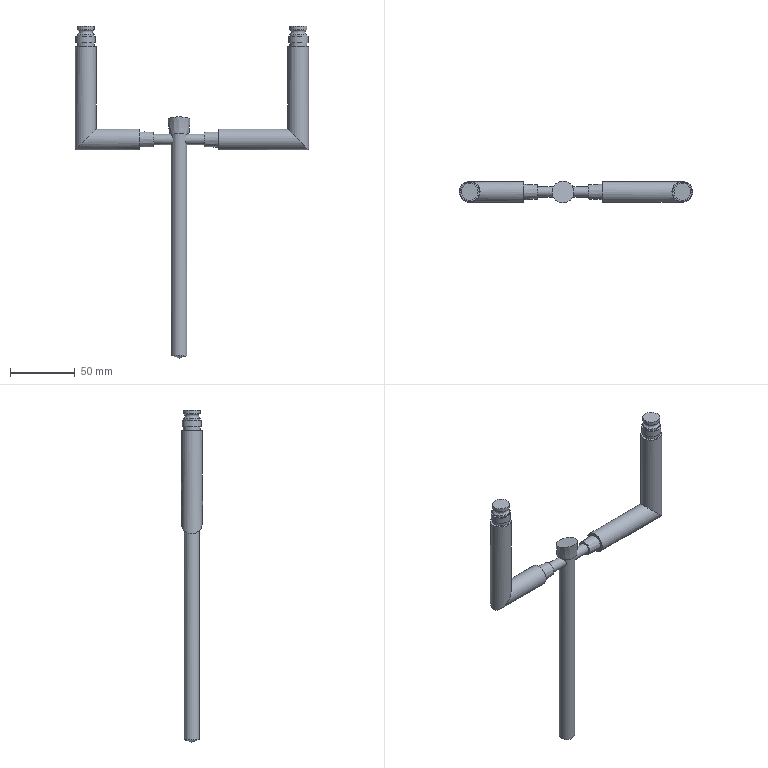Part | STEP file | COOLING-SLIDE2_id162_x_t | 1 solid | 35 faces | box 180 x 16.813 x 255.984 mm | volume 79230 mm3 | cylinder 15 | plane 14 | cone 4 | other 2 | commonest cylinder face diameters 13 x6 16 x4 8 x2 15 x2 12 x1
STEP:
#1=CARTESIAN_POINT('',(-95.5,0.,291.));
#2=VERTEX_POINT('',#1);
#3=CARTESIAN_POINT('',(-102.,0.,291.));
#4=DIRECTION('',(0.,0.,-1.));
#5=DIRECTION('',(1.,0.,0.));
#6=AXIS2_PLACEMENT_3D('',#3,#4,#5);
#7=CIRCLE('',#6,6.5);
#8=EDGE_CURVE('',#2,#2,#7,.T.);
#9=ORIENTED_EDGE('',*,*,#8,.F.);
#10=EDGE_LOOP('',(#9));
#11=FACE_OUTER_BOUND('',#10,.T.);
#12=CARTESIAN_POINT('',(-102.,0.,291.));
#13=DIRECTION('',(0.,0.,1.));
#14=DIRECTION('',(1.,0.,0.));
#15=AXIS2_PLACEMENT_3D('',#12,#13,#14);
#16=PLANE('',#15);
#17=ADVANCED_FACE('',(#11),#16,.T.);
#18=CARTESIAN_POINT('',(55.5,0.,291.));
#19=VERTEX_POINT('',#18);
#20=CARTESIAN_POINT('',(62.,0.,291.));
#21=DIRECTION('',(0.,0.,-1.));
#22=DIRECTION('',(-1.,0.,0.));
#23=AXIS2_PLACEMENT_3D('',#20,#21,#22);
#24=CIRCLE('',#23,6.5);
#25=EDGE_CURVE('',#19,#19,#24,.T.);
#26=ORIENTED_EDGE('',*,*,#25,.F.);
#27=EDGE_LOOP('',(#26));
#28=FACE_OUTER_BOUND('',#27,.T.);
#29=CARTESIAN_POINT('',(62.,0.,291.));
#30=DIRECTION('',(0.,0.,-1.));
#31=DIRECTION('',(-1.,0.,0.));
#32=AXIS2_PLACEMENT_3D('',#29,#30,#31);
#33=PLANE('',#32);
#34=ADVANCED_FACE('',(#28),#33,.F.);
#35=ORIENTED_EDGE('',*,*,#8,.T.);
#36=EDGE_LOOP('',(#35));
#37=FACE_BOUND('',#36,.T.);
#38=CARTESIAN_POINT('',(-108.5,0.,288.149));
#39=VERTEX_POINT('',#38);
#40=CARTESIAN_POINT('',(-102.,0.,288.149));
#41=DIRECTION('',(0.,0.,1.));
#42=DIRECTION('',(-1.,0.,0.));
#43=AXIS2_PLACEMENT_3D('',#40,#41,#42);
#44=CIRCLE('',#43,6.5);
#45=EDGE_CURVE('',#39,#39,#44,.T.);
#46=ORIENTED_EDGE('',*,*,#45,.T.);
#47=EDGE_LOOP('',(#46));
#48=FACE_BOUND('',#47,.T.);
#49=CARTESIAN_POINT('',(-102.,0.,190.725));
#50=DIRECTION('',(0.,0.,1.));
#51=DIRECTION('',(1.,0.,0.));
#52=AXIS2_PLACEMENT_3D('',#49,#50,#51);
#53=CYLINDRICAL_SURFACE('',#52,6.5);
#54=ADVANCED_FACE('',(#37,#48),#53,.T.);
#55=CARTESIAN_POINT('',(68.5,0.,288.149));
#56=VERTEX_POINT('',#55);
#57=CARTESIAN_POINT('',(62.,0.,288.149));
#58=DIRECTION('',(0.,0.,1.));
#59=DIRECTION('',(1.,0.,0.));
#60=AXIS2_PLACEMENT_3D('',#57,#58,#59);
#61=CIRCLE('',#60,6.5);
#62=EDGE_CURVE('',#56,#56,#61,.T.);
#63=ORIENTED_EDGE('',*,*,#62,.T.);
#64=EDGE_LOOP('',(#63));
#65=FACE_BOUND('',#64,.T.);
#66=ORIENTED_EDGE('',*,*,#25,.T.);
#67=EDGE_LOOP('',(#66));
#68=FACE_BOUND('',#67,.T.);
#69=CARTESIAN_POINT('',(62.,0.,295.775));
#70=DIRECTION('',(0.,0.,-1.));
#71=DIRECTION('',(-1.,0.,0.));
#72=AXIS2_PLACEMENT_3D('',#69,#70,#71);
#73=CYLINDRICAL_SURFACE('',#72,6.5);
#74=ADVANCED_FACE('',(#65,#68),#73,.T.);
#75=ORIENTED_EDGE('',*,*,#45,.F.);
#76=EDGE_LOOP('',(#75));
#77=FACE_BOUND('',#76,.T.);
#78=CARTESIAN_POINT('',(-95.5,0.,284.433));
#79=VERTEX_POINT('',#78);
#80=CARTESIAN_POINT('',(-102.,0.,284.433));
#81=DIRECTION('',(0.,0.,-1.));
#82=DIRECTION('',(1.,0.,0.));
#83=AXIS2_PLACEMENT_3D('',#80,#81,#82);
#84=CIRCLE('',#83,6.5);
#85=EDGE_CURVE('',#79,#79,#84,.T.);
#86=ORIENTED_EDGE('',*,*,#85,.F.);
#87=EDGE_LOOP('',(#86));
#88=FACE_BOUND('',#87,.T.);
#89=CARTESIAN_POINT('',(-109.241,0.,286.291));
#90=DIRECTION('',(0.,-1.,0.));
#91=DIRECTION('',(-1.,0.,0.));
#92=AXIS2_PLACEMENT_3D('',#89,#90,#91);
#93=CIRCLE('',#92,2.);
#94=CARTESIAN_POINT('',(-102.,0.,286.291));
#95=DIRECTION('',(0.,0.,1.));
#96=AXIS1_PLACEMENT('',#94,#95);
#97=SURFACE_OF_REVOLUTION('',#93,#96);
#98=ADVANCED_FACE('',(#77,#88),#97,.T.);
#99=CARTESIAN_POINT('',(55.5,0.,284.433));
#100=VERTEX_POINT('',#99);
#101=CARTESIAN_POINT('',(62.,0.,284.433));
#102=DIRECTION('',(0.,0.,-1.));
#103=DIRECTION('',(-1.,0.,0.));
#104=AXIS2_PLACEMENT_3D('',#101,#102,#103);
#105=CIRCLE('',#104,6.5);
#106=EDGE_CURVE('',#100,#100,#105,.T.);
#107=ORIENTED_EDGE('',*,*,#106,.F.);
#108=EDGE_LOOP('',(#107));
#109=FACE_BOUND('',#108,.T.);
#110=ORIENTED_EDGE('',*,*,#62,.F.);
#111=EDGE_LOOP('',(#110));
#112=FACE_BOUND('',#111,.T.);
#113=CARTESIAN_POINT('',(69.241,0.,286.291));
#114=DIRECTION('',(0.,-1.,0.));
#115=DIRECTION('',(1.,0.,0.));
#116=AXIS2_PLACEMENT_3D('',#113,#114,#115);
#117=CIRCLE('',#116,2.);
#118=CARTESIAN_POINT('',(62.,0.,286.291));
#119=DIRECTION('',(0.,0.,-1.));
#120=AXIS1_PLACEMENT('',#118,#119);
#121=SURFACE_OF_REVOLUTION('',#117,#120);
#122=ADVANCED_FACE('',(#109,#112),#121,.T.);
#123=ORIENTED_EDGE('',*,*,#85,.T.);
#124=EDGE_LOOP('',(#123));
#125=FACE_BOUND('',#124,.T.);
#126=CARTESIAN_POINT('',(-95.5,0.,283.));
#127=VERTEX_POINT('',#126);
#128=CARTESIAN_POINT('',(-102.,0.,283.));
#129=DIRECTION('',(0.,0.,-1.));
#130=DIRECTION('',(1.,0.,0.));
#131=AXIS2_PLACEMENT_3D('',#128,#129,#130);
#132=CIRCLE('',#131,6.5);
#133=EDGE_CURVE('',#127,#127,#132,.T.);
#134=ORIENTED_EDGE('',*,*,#133,.F.);
#135=EDGE_LOOP('',(#134));
#136=FACE_BOUND('',#135,.T.);
#137=CARTESIAN_POINT('',(-102.,0.,190.725));
#138=DIRECTION('',(0.,0.,1.));
#139=DIRECTION('',(1.,0.,0.));
#140=AXIS2_PLACEMENT_3D('',#137,#138,#139);
#141=CYLINDRICAL_SURFACE('',#140,6.5);
#142=ADVANCED_FACE('',(#125,#136),#141,.T.);
#143=CARTESIAN_POINT('',(55.5,0.,283.));
#144=VERTEX_POINT('',#143);
#145=CARTESIAN_POINT('',(62.,0.,283.));
#146=DIRECTION('',(0.,0.,1.));
#147=DIRECTION('',(-1.,0.,0.));
#148=AXIS2_PLACEMENT_3D('',#145,#146,#147);
#149=CIRCLE('',#148,6.5);
#150=EDGE_CURVE('',#144,#144,#149,.T.);
#151=ORIENTED_EDGE('',*,*,#150,.T.);
#152=EDGE_LOOP('',(#151));
#153=FACE_BOUND('',#152,.T.);
#154=ORIENTED_EDGE('',*,*,#106,.T.);
#155=EDGE_LOOP('',(#154));
#156=FACE_BOUND('',#155,.T.);
#157=CARTESIAN_POINT('',(62.,0.,295.775));
#158=DIRECTION('',(0.,0.,-1.));
#159=DIRECTION('',(-1.,0.,0.));
#160=AXIS2_PLACEMENT_3D('',#157,#158,#159);
#161=CYLINDRICAL_SURFACE('',#160,6.5);
#162=ADVANCED_FACE('',(#153,#156),#161,.T.);
#163=ORIENTED_EDGE('',*,*,#133,.T.);
#164=EDGE_LOOP('',(#163));
#165=FACE_BOUND('',#164,.T.);
#166=CARTESIAN_POINT('',(-94.5,0.,283.));
#167=VERTEX_POINT('',#166);
#168=CARTESIAN_POINT('',(-102.,0.,283.));
#169=DIRECTION('',(0.,0.,-1.));
#170=DIRECTION('',(1.,0.,0.));
#171=AXIS2_PLACEMENT_3D('',#168,#169,#170);
#172=CIRCLE('',#171,7.5);
#173=EDGE_CURVE('',#167,#167,#172,.T.);
#174=ORIENTED_EDGE('',*,*,#173,.F.);
#175=EDGE_LOOP('',(#174));
#176=FACE_BOUND('',#175,.T.);
#177=CARTESIAN_POINT('',(-102.,0.,283.));
#178=DIRECTION('',(0.,0.,1.));
#179=DIRECTION('',(1.,0.,0.));
#180=AXIS2_PLACEMENT_3D('',#177,#178,#179);
#181=PLANE('',#180);
#182=ADVANCED_FACE('',(#165,#176),#181,.T.);
#183=ORIENTED_EDGE('',*,*,#150,.F.);
#184=EDGE_LOOP('',(#183));
#185=FACE_BOUND('',#184,.T.);
#186=CARTESIAN_POINT('',(54.5,0.,283.));
#187=VERTEX_POINT('',#186);
#188=CARTESIAN_POINT('',(62.,0.,283.));
#189=DIRECTION('',(0.,0.,-1.));
#190=DIRECTION('',(-1.,0.,0.));
#191=AXIS2_PLACEMENT_3D('',#188,#189,#190);
#192=CIRCLE('',#191,7.5);
#193=EDGE_CURVE('',#187,#187,#192,.T.);
#194=ORIENTED_EDGE('',*,*,#193,.F.);
#195=EDGE_LOOP('',(#194));
#196=FACE_BOUND('',#195,.T.);
#197=CARTESIAN_POINT('',(62.,0.,283.));
#198=DIRECTION('',(0.,0.,-1.));
#199=DIRECTION('',(-1.,0.,0.));
#200=AXIS2_PLACEMENT_3D('',#197,#198,#199);
#201=PLANE('',#200);
#202=ADVANCED_FACE('',(#185,#196),#201,.F.);
#203=CARTESIAN_POINT('',(-94.5,0.,278.));
#204=VERTEX_POINT('',#203);
#205=CARTESIAN_POINT('',(-102.,0.,278.));
#206=DIRECTION('',(0.,0.,1.));
#207=DIRECTION('',(1.,0.,0.));
#208=AXIS2_PLACEMENT_3D('',#205,#206,#207);
#209=CIRCLE('',#208,7.5);
#210=EDGE_CURVE('',#204,#204,#209,.T.);
#211=ORIENTED_EDGE('',*,*,#210,.T.);
#212=EDGE_LOOP('',(#211));
#213=FACE_BOUND('',#212,.T.);
#214=ORIENTED_EDGE('',*,*,#173,.T.);
#215=EDGE_LOOP('',(#214));
#216=FACE_BOUND('',#215,.T.);
#217=CARTESIAN_POINT('',(-102.,0.,190.725));
#218=DIRECTION('',(0.,0.,1.));
#219=DIRECTION('',(1.,0.,0.));
#220=AXIS2_PLACEMENT_3D('',#217,#218,#219);
#221=CYLINDRICAL_SURFACE('',#220,7.5);
#222=ADVANCED_FACE('',(#213,#216),#221,.T.);
#223=ORIENTED_EDGE('',*,*,#193,.T.);
#224=EDGE_LOOP('',(#223));
#225=FACE_BOUND('',#224,.T.);
#226=CARTESIAN_POINT('',(54.5,0.,278.));
#227=VERTEX_POINT('',#226);
#228=CARTESIAN_POINT('',(62.,0.,278.));
#229=DIRECTION('',(0.,0.,-1.));
#230=DIRECTION('',(-1.,0.,0.));
#231=AXIS2_PLACEMENT_3D('',#228,#229,#230);
#232=CIRCLE('',#231,7.5);
#233=EDGE_CURVE('',#227,#227,#232,.T.);
#234=ORIENTED_EDGE('',*,*,#233,.F.);
#235=EDGE_LOOP('',(#234));
#236=FACE_BOUND('',#235,.T.);
#237=CARTESIAN_POINT('',(62.,0.,295.775));
#238=DIRECTION('',(0.,0.,-1.));
#239=DIRECTION('',(-1.,0.,0.));
#240=AXIS2_PLACEMENT_3D('',#237,#238,#239);
#241=CYLINDRICAL_SURFACE('',#240,7.5);
#242=ADVANCED_FACE('',(#225,#236),#241,.T.);
#243=CARTESIAN_POINT('',(-95.5,0.,278.));
#244=VERTEX_POINT('',#243);
#245=CARTESIAN_POINT('',(-102.,0.,278.));
#246=DIRECTION('',(0.,0.,-1.));
#247=DIRECTION('',(1.,0.,0.));
#248=AXIS2_PLACEMENT_3D('',#245,#246,#247);
#249=CIRCLE('',#248,6.5);
#250=EDGE_CURVE('',#244,#244,#249,.T.);
#251=ORIENTED_EDGE('',*,*,#250,.F.);
#252=EDGE_LOOP('',(#251));
#253=FACE_BOUND('',#252,.T.);
#254=ORIENTED_EDGE('',*,*,#210,.F.);
#255=EDGE_LOOP('',(#254));
#256=FACE_BOUND('',#255,.T.);
#257=CARTESIAN_POINT('',(-102.,0.,278.));
#258=DIRECTION('',(0.,0.,1.));
#259=DIRECTION('',(1.,0.,0.));
#260=AXIS2_PLACEMENT_3D('',#257,#258,#259);
#261=PLANE('',#260);
#262=ADVANCED_FACE('',(#253,#256),#261,.F.);
#263=CARTESIAN_POINT('',(55.5,0.,278.));
#264=VERTEX_POINT('',#263);
#265=CARTESIAN_POINT('',(62.,0.,278.));
#266=DIRECTION('',(0.,0.,-1.));
#267=DIRECTION('',(-1.,0.,0.));
#268=AXIS2_PLACEMENT_3D('',#265,#266,#267);
#269=CIRCLE('',#268,6.5);
#270=EDGE_CURVE('',#264,#264,#269,.T.);
#271=ORIENTED_EDGE('',*,*,#270,.F.);
#272=EDGE_LOOP('',(#271));
#273=FACE_BOUND('',#272,.T.);
#274=ORIENTED_EDGE('',*,*,#233,.T.);
#275=EDGE_LOOP('',(#274));
#276=FACE_BOUND('',#275,.T.);
#277=CARTESIAN_POINT('',(62.,0.,278.));
#278=DIRECTION('',(0.,0.,-1.));
#279=DIRECTION('',(-1.,0.,0.));
#280=AXIS2_PLACEMENT_3D('',#277,#278,#279);
#281=PLANE('',#280);
#282=ADVANCED_FACE('',(#273,#276),#281,.T.);
#283=ORIENTED_EDGE('',*,*,#250,.T.);
#284=EDGE_LOOP('',(#283));
#285=FACE_BOUND('',#284,.T.);
#286=CARTESIAN_POINT('',(-95.5,0.,275.));
#287=VERTEX_POINT('',#286);
#288=CARTESIAN_POINT('',(-102.,0.,275.));
#289=DIRECTION('',(0.,0.,-1.));
#290=DIRECTION('',(1.,0.,0.));
#291=AXIS2_PLACEMENT_3D('',#288,#289,#290);
#292=CIRCLE('',#291,6.5);
#293=EDGE_CURVE('',#287,#287,#292,.T.);
#294=ORIENTED_EDGE('',*,*,#293,.F.);
#295=EDGE_LOOP('',(#294));
#296=FACE_BOUND('',#295,.T.);
#297=CARTESIAN_POINT('',(-102.,0.,190.725));
#298=DIRECTION('',(0.,0.,1.));
#299=DIRECTION('',(1.,0.,0.));
#300=AXIS2_PLACEMENT_3D('',#297,#298,#299);
#301=CYLINDRICAL_SURFACE('',#300,6.5);
#302=ADVANCED_FACE('',(#285,#296),#301,.T.);
#303=CARTESIAN_POINT('',(55.5,0.,275.));
#304=VERTEX_POINT('',#303);
#305=CARTESIAN_POINT('',(62.,0.,275.));
#306=DIRECTION('',(0.,0.,1.));
#307=DIRECTION('',(-1.,0.,0.));
#308=AXIS2_PLACEMENT_3D('',#305,#306,#307);
#309=CIRCLE('',#308,6.5);
#310=EDGE_CURVE('',#304,#304,#309,.T.);
#311=ORIENTED_EDGE('',*,*,#310,.T.);
#312=EDGE_LOOP('',(#311));
#313=FACE_BOUND('',#312,.T.);
#314=ORIENTED_EDGE('',*,*,#270,.T.);
#315=EDGE_LOOP('',(#314));
#316=FACE_BOUND('',#315,.T.);
#317=CARTESIAN_POINT('',(62.,0.,295.775));
#318=DIRECTION('',(0.,0.,-1.));
#319=DIRECTION('',(-1.,0.,0.));
#320=AXIS2_PLACEMENT_3D('',#317,#318,#319);
#321=CYLINDRICAL_SURFACE('',#320,6.5);
#322=ADVANCED_FACE('',(#313,#316),#321,.T.);
#323=ORIENTED_EDGE('',*,*,#293,.T.);
#324=EDGE_LOOP('',(#323));
#325=FACE_BOUND('',#324,.T.);
#326=CARTESIAN_POINT('',(-94.,0.,275.));
#327=VERTEX_POINT('',#326);
#328=CARTESIAN_POINT('',(-102.,0.,275.));
#329=DIRECTION('',(0.,0.,-1.));
#330=DIRECTION('',(1.,0.,0.));
#331=AXIS2_PLACEMENT_3D('',#328,#329,#330);
#332=CIRCLE('',#331,8.);
#333=EDGE_CURVE('',#327,#327,#332,.T.);
#334=ORIENTED_EDGE('',*,*,#333,.F.);
#335=EDGE_LOOP('',(#334));
#336=FACE_BOUND('',#335,.T.);
#337=CARTESIAN_POINT('',(-102.,0.,275.));
#338=DIRECTION('',(0.,0.,1.));
#339=DIRECTION('',(1.,0.,0.));
#340=AXIS2_PLACEMENT_3D('',#337,#338,#339);
#341=PLANE('',#340);
#342=ADVANCED_FACE('',(#325,#336),#341,.T.);
#343=ORIENTED_EDGE('',*,*,#310,.F.);
#344=EDGE_LOOP('',(#343));
#345=FACE_BOUND('',#344,.T.);
#346=CARTESIAN_POINT('',(54.,0.,275.));
#347=VERTEX_POINT('',#346);
#348=CARTESIAN_POINT('',(62.,0.,275.));
#349=DIRECTION('',(0.,0.,-1.));
#350=DIRECTION('',(-1.,0.,0.));
#351=AXIS2_PLACEMENT_3D('',#348,#349,#350);
#352=CIRCLE('',#351,8.);
#353=EDGE_CURVE('',#347,#347,#352,.T.);
#354=ORIENTED_EDGE('',*,*,#353,.F.);
#355=EDGE_LOOP('',(#354));
#356=FACE_BOUND('',#355,.T.);
#357=CARTESIAN_POINT('',(62.,0.,275.));
#358=DIRECTION('',(0.,0.,-1.));
#359=DIRECTION('',(-1.,0.,0.));
#360=AXIS2_PLACEMENT_3D('',#357,#358,#359);
#361=PLANE('',#360);
#362=ADVANCED_FACE('',(#345,#356),#361,.F.);
#363=ORIENTED_EDGE('',*,*,#333,.T.);
#364=EDGE_LOOP('',(#363));
#365=FACE_BOUND('',#364,.T.);
#366=CARTESIAN_POINT('',(-110.,0.,195.5));
#367=VERTEX_POINT('',#366);
#368=CARTESIAN_POINT('',(-102.,0.,203.5));
#369=DIRECTION('',(0.7071,0.,-0.7071));
#370=DIRECTION('',(-0.7071,0.,-0.7071));
#371=AXIS2_PLACEMENT_3D('',#368,#369,#370);
#372=ELLIPSE('',#371,11.314,8.);
#373=EDGE_CURVE('',#367,#367,#372,.T.);
#374=ORIENTED_EDGE('',*,*,#373,.F.);
#375=EDGE_LOOP('',(#374));
#376=FACE_BOUND('',#375,.T.);
#377=CARTESIAN_POINT('',(-102.,0.,190.725));
#378=DIRECTION('',(0.,0.,1.));
#379=DIRECTION('',(1.,0.,0.));
#380=AXIS2_PLACEMENT_3D('',#377,#378,#379);
#381=CYLINDRICAL_SURFACE('',#380,8.);
#382=ADVANCED_FACE('',(#365,#376),#381,.T.);
#383=ORIENTED_EDGE('',*,*,#353,.T.);
#384=EDGE_LOOP('',(#383));
#385=FACE_BOUND('',#384,.T.);
#386=CARTESIAN_POINT('',(54.,0.,211.5));
#387=VERTEX_POINT('',#386);
#388=CARTESIAN_POINT('',(62.,0.,203.5));
#389=DIRECTION('',(-0.7071,0.,-0.7071));
#390=DIRECTION('',(-0.7071,0.,0.7071));
#391=AXIS2_PLACEMENT_3D('',#388,#389,#390);
#392=ELLIPSE('',#391,11.314,8.);
#393=EDGE_CURVE('',#387,#387,#392,.T.);
#394=ORIENTED_EDGE('',*,*,#393,.F.);
#395=EDGE_LOOP('',(#394));
#396=FACE_BOUND('',#395,.T.);
#397=CARTESIAN_POINT('',(62.,0.,295.775));
#398=DIRECTION('',(0.,0.,-1.));
#399=DIRECTION('',(-1.,0.,0.));
#400=AXIS2_PLACEMENT_3D('',#397,#398,#399);
#401=CYLINDRICAL_SURFACE('',#400,8.);
#402=ADVANCED_FACE('',(#385,#396),#401,.T.);
#403=CARTESIAN_POINT('',(-60.5,0.,211.5));
#404=VERTEX_POINT('',#403);
#405=CARTESIAN_POINT('',(-60.5,0.,203.5));
#406=DIRECTION('',(-1.,0.,0.));
#407=DIRECTION('',(0.,0.,1.));
#408=AXIS2_PLACEMENT_3D('',#405,#406,#407);
#409=CIRCLE('',#408,8.);
#410=EDGE_CURVE('',#404,#404,#409,.T.);
#411=ORIENTED_EDGE('',*,*,#410,.T.);
#412=EDGE_LOOP('',(#411));
#413=FACE_BOUND('',#412,.T.);
#414=ORIENTED_EDGE('',*,*,#373,.T.);
#415=EDGE_LOOP('',(#414));
#416=FACE_BOUND('',#415,.T.);
#417=CARTESIAN_POINT('',(79.,0.,203.5));
#418=DIRECTION('',(-1.,0.,0.));
#419=DIRECTION('',(0.,0.,1.));
#420=AXIS2_PLACEMENT_3D('',#417,#418,#419);
#421=CYLINDRICAL_SURFACE('',#420,8.);
#422=ADVANCED_FACE('',(#413,#416),#421,.T.);
#423=CARTESIAN_POINT('',(0.5,0.,211.5));
#424=VERTEX_POINT('',#423);
#425=CARTESIAN_POINT('',(0.5,0.,203.5));
#426=DIRECTION('',(-1.,0.,0.));
#427=DIRECTION('',(0.,0.,1.));
#428=AXIS2_PLACEMENT_3D('',#425,#426,#427);
#429=CIRCLE('',#428,8.);
#430=EDGE_CURVE('',#424,#424,#429,.T.);
#431=ORIENTED_EDGE('',*,*,#430,.F.);
#432=EDGE_LOOP('',(#431));
#433=FACE_BOUND('',#432,.T.);
#434=ORIENTED_EDGE('',*,*,#393,.T.);
#435=EDGE_LOOP('',(#434));
#436=FACE_BOUND('',#435,.T.);
#437=CARTESIAN_POINT('',(79.,0.,203.5));
#438=DIRECTION('',(-1.,0.,0.));
#439=DIRECTION('',(0.,0.,1.));
#440=AXIS2_PLACEMENT_3D('',#437,#438,#439);
#441=CYLINDRICAL_SURFACE('',#440,8.);
#442=ADVANCED_FACE('',(#433,#436),#441,.T.);
#443=CARTESIAN_POINT('',(-60.5,-6.,203.5));
#444=VERTEX_POINT('',#443);
#445=CARTESIAN_POINT('',(-60.5,0.,203.5));
#446=DIRECTION('',(1.,0.,0.));
#447=DIRECTION('',(0.,-1.,0.));
#448=AXIS2_PLACEMENT_3D('',#445,#446,#447);
#449=CIRCLE('',#448,6.);
#450=EDGE_CURVE('',#444,#444,#449,.T.);
#451=ORIENTED_EDGE('',*,*,#450,.F.);
#452=EDGE_LOOP('',(#451));
#453=FACE_BOUND('',#452,.T.);
#454=ORIENTED_EDGE('',*,*,#410,.F.);
#455=EDGE_LOOP('',(#454));
#456=FACE_BOUND('',#455,.T.);
#457=CARTESIAN_POINT('',(-60.5,0.,203.5));
#458=DIRECTION('',(-1.,0.,0.));
#459=DIRECTION('',(0.,0.,1.));
#460=AXIS2_PLACEMENT_3D('',#457,#458,#459);
#461=PLANE('',#460);
#462=ADVANCED_FACE('',(#453,#456),#461,.F.);
#463=CARTESIAN_POINT('',(0.5,0.,197.5));
#464=VERTEX_POINT('',#463);
#465=CARTESIAN_POINT('',(0.5,0.,203.5));
#466=DIRECTION('',(-1.,0.,0.));
#467=DIRECTION('',(0.,0.,-1.));
#468=AXIS2_PLACEMENT_3D('',#465,#466,#467);
#469=CIRCLE('',#468,6.);
#470=EDGE_CURVE('',#464,#464,#469,.T.);
#471=ORIENTED_EDGE('',*,*,#470,.F.);
#472=EDGE_LOOP('',(#471));
#473=FACE_BOUND('',#472,.T.);
#474=ORIENTED_EDGE('',*,*,#430,.T.);
#475=EDGE_LOOP('',(#474));
#476=FACE_BOUND('',#475,.T.);
#477=CARTESIAN_POINT('',(0.5,0.,203.5));
#478=DIRECTION('',(-1.,0.,0.));
#479=DIRECTION('',(0.,0.,1.));
#480=AXIS2_PLACEMENT_3D('',#477,#478,#479);
#481=PLANE('',#480);
#482=ADVANCED_FACE('',(#473,#476),#481,.T.);
#483=CARTESIAN_POINT('',(-30.,-8.535,220.974));
#484=VERTEX_POINT('',#483);
#485=CARTESIAN_POINT('',(-30.,-0.1282,218.878));
#486=DIRECTION('',(0.,-0.2419,-0.9703));
#487=DIRECTION('',(0.,-0.9703,0.2419));
#488=AXIS2_PLACEMENT_3D('',#485,#486,#487);
#489=ELLIPSE('',#488,8.664,8.406);
#490=EDGE_CURVE('',#484,#484,#489,.T.);
#491=ORIENTED_EDGE('',*,*,#490,.F.);
#492=EDGE_LOOP('',(#491));
#493=FACE_OUTER_BOUND('',#492,.T.);
#494=CARTESIAN_POINT('',(-90.,-21.1,224.107));
#495=DIRECTION('',(0.,-0.2419,-0.9703));
#496=DIRECTION('',(0.,0.9703,-0.2419));
#497=AXIS2_PLACEMENT_3D('',#494,#495,#496);
#498=PLANE('',#497);
#499=ADVANCED_FACE('',(#493),#498,.F.);
#500=CARTESIAN_POINT('',(-49.5,-5.5,203.5));
#501=VERTEX_POINT('',#500);
#502=CARTESIAN_POINT('',(-49.5,0.,203.5));
#503=DIRECTION('',(-1.,0.,0.));
#504=DIRECTION('',(0.,-1.,0.));
#505=AXIS2_PLACEMENT_3D('',#502,#503,#504);
#506=CIRCLE('',#505,5.5);
#507=EDGE_CURVE('',#501,#501,#506,.T.);
#508=ORIENTED_EDGE('',*,*,#507,.T.);
#509=EDGE_LOOP('',(#508));
#510=FACE_BOUND('',#509,.T.);
#511=ORIENTED_EDGE('',*,*,#450,.T.);
#512=EDGE_LOOP('',(#511));
#513=FACE_BOUND('',#512,.T.);
#514=CARTESIAN_POINT('',(-60.5,0.,203.5));
#515=DIRECTION('',(-1.,0.,0.));
#516=DIRECTION('',(0.,-1.,0.));
#517=AXIS2_PLACEMENT_3D('',#514,#515,#516);
#518=CONICAL_SURFACE('',#517,6.,2.603);
#519=ADVANCED_FACE('',(#510,#513),#518,.T.);
#520=ORIENTED_EDGE('',*,*,#470,.T.);
#521=EDGE_LOOP('',(#520));
#522=FACE_BOUND('',#521,.T.);
#523=CARTESIAN_POINT('',(-10.5,0.,198.));
#524=VERTEX_POINT('',#523);
#525=CARTESIAN_POINT('',(-10.5,0.,203.5));
#526=DIRECTION('',(-1.,0.,0.));
#527=DIRECTION('',(0.,0.,-1.));
#528=AXIS2_PLACEMENT_3D('',#525,#526,#527);
#529=CIRCLE('',#528,5.5);
#530=EDGE_CURVE('',#524,#524,#529,.T.);
#531=ORIENTED_EDGE('',*,*,#530,.F.);
#532=EDGE_LOOP('',(#531));
#533=FACE_BOUND('',#532,.T.);
#534=CARTESIAN_POINT('',(0.5,0.,203.5));
#535=DIRECTION('',(1.,0.,0.));
#536=DIRECTION('',(0.,0.,-1.));
#537=AXIS2_PLACEMENT_3D('',#534,#535,#536);
#538=CONICAL_SURFACE('',#537,6.,2.603);
#539=ADVANCED_FACE('',(#522,#533),#538,.T.);
#540=CARTESIAN_POINT('',(-30.,-7.741,208.));
#541=VERTEX_POINT('',#540);
#542=CARTESIAN_POINT('',(-30.,0.,208.));
#543=DIRECTION('',(0.,0.,-1.));
#544=DIRECTION('',(0.,-1.,0.));
#545=AXIS2_PLACEMENT_3D('',#542,#543,#544);
#546=CIRCLE('',#545,7.741);
#547=EDGE_CURVE('',#541,#541,#546,.T.);
#548=ORIENTED_EDGE('',*,*,#547,.F.);
#549=EDGE_LOOP('',(#548));
#550=FACE_BOUND('',#549,.T.);
#551=ORIENTED_EDGE('',*,*,#490,.T.);
#552=EDGE_LOOP('',(#551));
#553=FACE_BOUND('',#552,.T.);
#554=CARTESIAN_POINT('',(-30.,0.,218.911));
#555=DIRECTION('',(0.,0.,1.));
#556=DIRECTION('',(0.,-1.,0.));
#557=AXIS2_PLACEMENT_3D('',#554,#555,#556);
#558=CONICAL_SURFACE('',#557,8.409,3.5);
#559=ADVANCED_FACE('',(#550,#553),#558,.T.);
#560=CARTESIAN_POINT('',(-49.5,0.,207.5));
#561=VERTEX_POINT('',#560);
#562=CARTESIAN_POINT('',(-49.5,0.,203.5));
#563=DIRECTION('',(1.,0.,0.));
#564=DIRECTION('',(0.,0.,1.));
#565=AXIS2_PLACEMENT_3D('',#562,#563,#564);
#566=CIRCLE('',#565,4.);
#567=EDGE_CURVE('',#561,#561,#566,.T.);
#568=ORIENTED_EDGE('',*,*,#567,.F.);
#569=EDGE_LOOP('',(#568));
#570=FACE_BOUND('',#569,.T.);
#571=ORIENTED_EDGE('',*,*,#507,.F.);
#572=EDGE_LOOP('',(#571));
#573=FACE_BOUND('',#572,.T.);
#574=CARTESIAN_POINT('',(-49.5,0.,203.5));
#575=DIRECTION('',(-1.,0.,0.));
#576=DIRECTION('',(0.,0.,1.));
#577=AXIS2_PLACEMENT_3D('',#574,#575,#576);
#578=PLANE('',#577);
#579=ADVANCED_FACE('',(#570,#573),#578,.F.);
#580=CARTESIAN_POINT('',(-10.5,0.,207.5));
#581=VERTEX_POINT('',#580);
#582=CARTESIAN_POINT('',(-10.5,0.,203.5));
#583=DIRECTION('',(-1.,0.,0.));
#584=DIRECTION('',(0.,0.,1.));
#585=AXIS2_PLACEMENT_3D('',#582,#583,#584);
#586=CIRCLE('',#585,4.);
#587=EDGE_CURVE('',#581,#581,#586,.T.);
#588=ORIENTED_EDGE('',*,*,#587,.F.);
#589=EDGE_LOOP('',(#588));
#590=FACE_BOUND('',#589,.T.);
#591=ORIENTED_EDGE('',*,*,#530,.T.);
#592=EDGE_LOOP('',(#591));
#593=FACE_BOUND('',#592,.T.);
#594=CARTESIAN_POINT('',(-10.5,0.,203.5));
#595=DIRECTION('',(-1.,0.,0.));
#596=DIRECTION('',(0.,0.,1.));
#597=AXIS2_PLACEMENT_3D('',#594,#595,#596);
#598=PLANE('',#597);
#599=ADVANCED_FACE('',(#590,#593),#598,.T.);
#600=CARTESIAN_POINT('',(-36.,0.,208.));
#601=VERTEX_POINT('',#600);
#602=CARTESIAN_POINT('',(-30.,0.,208.));
#603=DIRECTION('',(0.,0.,-1.));
#604=DIRECTION('',(-1.,0.,0.));
#605=AXIS2_PLACEMENT_3D('',#602,#603,#604);
#606=CIRCLE('',#605,6.);
#607=EDGE_CURVE('',#601,#601,#606,.T.);
#608=ORIENTED_EDGE('',*,*,#607,.F.);
#609=EDGE_LOOP('',(#608));
#610=FACE_BOUND('',#609,.T.);
#611=ORIENTED_EDGE('',*,*,#547,.T.);
#612=EDGE_LOOP('',(#611));
#613=FACE_BOUND('',#612,.T.);
#614=CARTESIAN_POINT('',(-30.,0.,208.));
#615=DIRECTION('',(0.,0.,-1.));
#616=DIRECTION('',(-1.,0.,0.));
#617=AXIS2_PLACEMENT_3D('',#614,#615,#616);
#618=PLANE('',#617);
#619=ADVANCED_FACE('',(#610,#613),#618,.T.);
#620=ORIENTED_EDGE('',*,*,#567,.T.);
#621=EDGE_LOOP('',(#620));
#622=FACE_BOUND('',#621,.T.);
#623=CARTESIAN_POINT('',(-36.,0.,207.5));
#624=VERTEX_POINT('',#623);
#625=CARTESIAN_POINT('',(-36.,1.093,207.5));
#626=CARTESIAN_POINT('',(-36.,-1.093,207.5));
#627=CARTESIAN_POINT('',(-35.671,-2.12,207.039));
#628=CARTESIAN_POINT('',(-34.907,-3.546,205.608));
#629=CARTESIAN_POINT('',(-34.475,-3.997,204.596));
#630=CARTESIAN_POINT('',(-34.469,-4.003,202.427));
#631=CARTESIAN_POINT('',(-34.898,-3.559,201.41));
#632=CARTESIAN_POINT('',(-35.668,-2.129,199.964));
#633=CARTESIAN_POINT('',(-35.998,-1.105,199.503));
#634=CARTESIAN_POINT('',(-36.002,1.084,199.497));
#635=CARTESIAN_POINT('',(-35.673,2.115,199.957));
#636=CARTESIAN_POINT('',(-34.908,3.545,201.389));
#637=CARTESIAN_POINT('',(-34.475,3.997,202.402));
#638=CARTESIAN_POINT('',(-34.469,4.003,204.575));
#639=CARTESIAN_POINT('',(-34.9,3.558,205.593));
#640=CARTESIAN_POINT('',(-35.67,2.123,207.04));
#641=CARTESIAN_POINT('',(-36.,1.093,207.5));
#642=CARTESIAN_POINT('',(-36.,-1.093,207.5));
#643=B_SPLINE_CURVE_WITH_KNOTS('',3,(#625,#626,#627,#628,#629,#630,#631,#632,#633,#634,#635,#636,#637,#638,#639,#640,#641,#642),.UNSPECIFIED.,.T.,.F.,(2,2,2,2,2,2,2,2,2,2,2),(-0.125,0.,0.125,0.25,0.375,0.5,0.625,0.75,0.875,1.,1.125),.UNSPECIFIED.);
#644=EDGE_CURVE('',#624,#624,#643,.T.);
#645=ORIENTED_EDGE('',*,*,#644,.F.);
#646=EDGE_LOOP('',(#645));
#647=FACE_BOUND('',#646,.T.);
#648=CARTESIAN_POINT('',(79.,0.,203.5));
#649=DIRECTION('',(-1.,0.,0.));
#650=DIRECTION('',(0.,0.,1.));
#651=AXIS2_PLACEMENT_3D('',#648,#649,#650);
#652=CYLINDRICAL_SURFACE('',#651,4.);
#653=ADVANCED_FACE('',(#622,#647),#652,.T.);
#654=CARTESIAN_POINT('',(-30.,0.,35.016));
#655=VERTEX_POINT('',#654);
#656=VERTEX_LOOP('',#655);
#657=FACE_BOUND('',#656,.T.);
#658=CARTESIAN_POINT('',(-36.,0.,36.782));
#659=VERTEX_POINT('',#658);
#660=CARTESIAN_POINT('',(-30.,0.,36.782));
#661=DIRECTION('',(0.,0.,1.));
#662=DIRECTION('',(-1.,0.,0.));
#663=AXIS2_PLACEMENT_3D('',#660,#661,#662);
#664=CIRCLE('',#663,6.);
#665=EDGE_CURVE('',#659,#659,#664,.T.);
#666=ORIENTED_EDGE('',*,*,#665,.F.);
#667=EDGE_LOOP('',(#666));
#668=FACE_BOUND('',#667,.T.);
#669=CARTESIAN_POINT('',(-30.,0.,36.782));
#670=DIRECTION('',(0.,0.,1.));
#671=DIRECTION('',(1.,0.,0.));
#672=AXIS2_PLACEMENT_3D('',#669,#670,#671);
#673=CONICAL_SURFACE('',#672,6.,73.607);
#674=ADVANCED_FACE('',(#657,#668),#673,.T.);
#675=ORIENTED_EDGE('',*,*,#587,.T.);
#676=EDGE_LOOP('',(#675));
#677=FACE_BOUND('',#676,.T.);
#678=CARTESIAN_POINT('',(-24.,0.,199.5));
#679=VERTEX_POINT('',#678);
#680=CARTESIAN_POINT('',(-24.,1.093,199.5));
#681=CARTESIAN_POINT('',(-24.,-1.093,199.5));
#682=CARTESIAN_POINT('',(-24.329,-2.12,199.961));
#683=CARTESIAN_POINT('',(-25.093,-3.546,201.392));
#684=CARTESIAN_POINT('',(-25.525,-3.997,202.404));
#685=CARTESIAN_POINT('',(-25.531,-4.003,204.573));
#686=CARTESIAN_POINT('',(-25.102,-3.559,205.59));
#687=CARTESIAN_POINT('',(-24.332,-2.129,207.036));
#688=CARTESIAN_POINT('',(-24.002,-1.105,207.497));
#689=CARTESIAN_POINT('',(-23.998,1.084,207.503));
#690=CARTESIAN_POINT('',(-24.327,2.115,207.043));
#691=CARTESIAN_POINT('',(-25.092,3.545,205.611));
#692=CARTESIAN_POINT('',(-25.525,3.997,204.598));
#693=CARTESIAN_POINT('',(-25.531,4.003,202.425));
#694=CARTESIAN_POINT('',(-25.1,3.558,201.407));
#695=CARTESIAN_POINT('',(-24.33,2.123,199.96));
#696=CARTESIAN_POINT('',(-24.,1.093,199.5));
#697=CARTESIAN_POINT('',(-24.,-1.093,199.5));
#698=B_SPLINE_CURVE_WITH_KNOTS('',3,(#680,#681,#682,#683,#684,#685,#686,#687,#688,#689,#690,#691,#692,#693,#694,#695,#696,#697),.UNSPECIFIED.,.T.,.F.,(2,2,2,2,2,2,2,2,2,2,2),(-0.125,0.,0.125,0.25,0.375,0.5,0.625,0.75,0.875,1.,1.125),.UNSPECIFIED.);
#699=EDGE_CURVE('',#679,#679,#698,.T.);
#700=ORIENTED_EDGE('',*,*,#699,.F.);
#701=EDGE_LOOP('',(#700));
#702=FACE_BOUND('',#701,.T.);
#703=CARTESIAN_POINT('',(79.,0.,203.5));
#704=DIRECTION('',(-1.,0.,0.));
#705=DIRECTION('',(0.,0.,1.));
#706=AXIS2_PLACEMENT_3D('',#703,#704,#705);
#707=CYLINDRICAL_SURFACE('',#706,4.);
#708=ADVANCED_FACE('',(#677,#702),#707,.T.);
#709=ORIENTED_EDGE('',*,*,#607,.T.);
#710=EDGE_LOOP('',(#709));
#711=FACE_BOUND('',#710,.T.);
#712=ORIENTED_EDGE('',*,*,#644,.T.);
#713=EDGE_LOOP('',(#712));
#714=FACE_BOUND('',#713,.T.);
#715=ORIENTED_EDGE('',*,*,#665,.T.);
#716=EDGE_LOOP('',(#715));
#717=FACE_BOUND('',#716,.T.);
#718=ORIENTED_EDGE('',*,*,#699,.T.);
#719=EDGE_LOOP('',(#718));
#720=FACE_BOUND('',#719,.T.);
#721=CARTESIAN_POINT('',(-30.,0.,236.022));
#722=DIRECTION('',(0.,0.,-1.));
#723=DIRECTION('',(-1.,0.,0.));
#724=AXIS2_PLACEMENT_3D('',#721,#722,#723);
#725=CYLINDRICAL_SURFACE('',#724,6.);
#726=ADVANCED_FACE('',(#711,#714,#717,#720),#725,.T.);
#727=CLOSED_SHELL('',(#17,#34,#54,#74,#98,#122,#142,#162,#182,#202,#222,#242,#262,#282,#302,#322,#342,#362,#382,#402,#422,#442,#462,#482,#499,#519,#539,#559,#579,#599,#619,#653,#674,#708,#726));
#728=MANIFOLD_SOLID_BREP('',#727);
#729=(LENGTH_UNIT()NAMED_UNIT(*)SI_UNIT(.MILLI.,.METRE.));
#730=UNCERTAINTY_MEASURE_WITH_UNIT(LENGTH_MEASURE(0.0508),#729,'','');
#731=(NAMED_UNIT(*)PLANE_ANGLE_UNIT()SI_UNIT($,.RADIAN.));
#732=PLANE_ANGLE_MEASURE_WITH_UNIT(PLANE_ANGLE_MEASURE(0.01745),#731);
#733=DIMENSIONAL_EXPONENTS(0.,0.,0.,0.,0.,0.,0.);
#734=(CONVERSION_BASED_UNIT('DEGREE',#732)NAMED_UNIT(#733)PLANE_ANGLE_UNIT());
#735=(NAMED_UNIT(*)SI_UNIT($,.STERADIAN.)SOLID_ANGLE_UNIT());
#736=(GEOMETRIC_REPRESENTATION_CONTEXT(3)GLOBAL_UNCERTAINTY_ASSIGNED_CONTEXT((#730))GLOBAL_UNIT_ASSIGNED_CONTEXT((#729,#734,#735))REPRESENTATION_CONTEXT('',''));
#737=ADVANCED_BREP_SHAPE_REPRESENTATION('',(#728),#736);